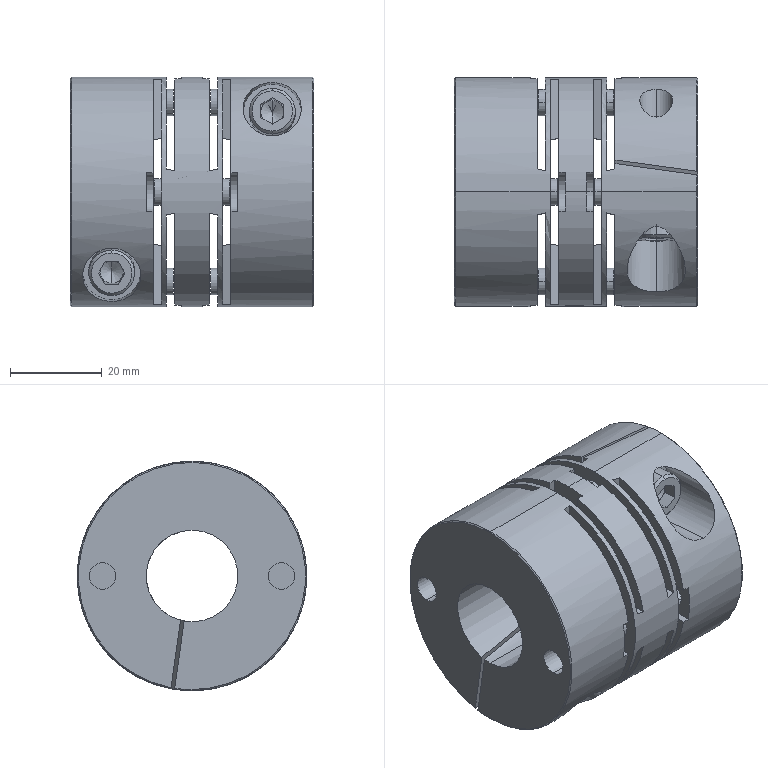Part | SolidWorks | 3 solids | 207 faces | box 53 x 50 x 50 mm | volume 69977 mm3 | plane 105 | cylinder 72 | cone 26 | torus 4 | commonest cylinder face diameters 5.8 x24 8.5 x10 4.917 x8 6 x8 20 x6 7.2 x4